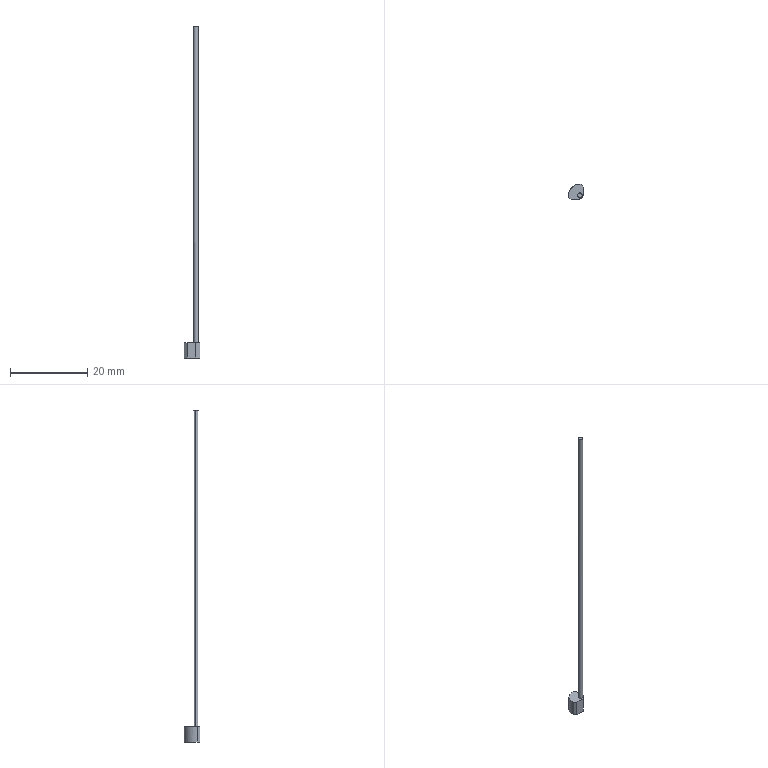Part | Creo | 1 solid | 13 faces | box 4 x 4 x 86.149 mm | volume 144.445 mm3 | plane 8 | cylinder 3 | cone 2 | commonest cylinder face diameters 1.2 x2 6 x1
STEP:
#1=CARTESIAN_POINT('',(0.,0.,0.));
#2=DIRECTION('',(0.,0.,1.));
#3=DIRECTION('',(1.,0.,0.));
#4=AXIS2_PLACEMENT_3D('',#1,#2,#3);
#5=CARTESIAN_POINT('',(29.569,-76.905,32.05));
#6=VERTEX_POINT('',#5);
#7=CARTESIAN_POINT('',(28.969,-77.496,32.059));
#8=VERTEX_POINT('',#7);
#9=CARTESIAN_POINT('',(29.569,-77.496,32.059));
#10=DIRECTION('',(0.,0.,1.));
#11=DIRECTION('',(-0.000001887,1.,0.));
#12=AXIS2_PLACEMENT_3D('',#9,#10,#11);
#13=CIRCLE('',#12,0.6);
#14=EDGE_CURVE('',#6,#8,#13,.T.);
#15=ORIENTED_EDGE('',*,*,#14,.T.);
#16=CARTESIAN_POINT('',(28.969,-77.496,-50.09));
#17=VERTEX_POINT('',#16);
#18=CARTESIAN_POINT('',(28.969,-77.496,32.059));
#19=DIRECTION('',(0.,0.,-1.));
#20=VECTOR('',#19,82.149);
#21=LINE('',#18,#20);
#22=EDGE_CURVE('',#8,#17,#21,.T.);
#23=ORIENTED_EDGE('',*,*,#22,.T.);
#24=CARTESIAN_POINT('',(30.169,-77.496,-50.09));
#25=VERTEX_POINT('',#24);
#26=CARTESIAN_POINT('',(29.569,-77.496,-50.09));
#27=DIRECTION('',(0.,0.,-1.));
#28=DIRECTION('',(-1.,0.,0.));
#29=AXIS2_PLACEMENT_3D('',#26,#27,#28);
#30=CIRCLE('',#29,0.6);
#31=EDGE_CURVE('',#17,#25,#30,.T.);
#32=ORIENTED_EDGE('',*,*,#31,.T.);
#33=CARTESIAN_POINT('',(30.169,-77.496,32.059));
#34=VERTEX_POINT('',#33);
#35=CARTESIAN_POINT('',(30.169,-77.496,32.059));
#36=DIRECTION('',(0.,0.,-1.));
#37=VECTOR('',#36,82.149);
#38=LINE('',#35,#37);
#39=EDGE_CURVE('',#34,#25,#38,.T.);
#40=ORIENTED_EDGE('',*,*,#39,.F.);
#41=CARTESIAN_POINT('',(29.569,-77.496,32.059));
#42=DIRECTION('',(0.,0.,1.));
#43=DIRECTION('',(1.,0.,0.));
#44=AXIS2_PLACEMENT_3D('',#41,#42,#43);
#45=CIRCLE('',#44,0.6);
#46=EDGE_CURVE('',#34,#6,#45,.T.);
#47=ORIENTED_EDGE('',*,*,#46,.T.);
#48=EDGE_LOOP('',(#15,#23,#32,#40,#47));
#49=FACE_OUTER_BOUND('',#48,.F.);
#50=CARTESIAN_POINT('',(29.569,-77.496,32.041));
#51=DIRECTION('',(0.,0.,-1.));
#52=DIRECTION('',(-1.,0.,0.));
#53=AXIS2_PLACEMENT_3D('',#50,#51,#52);
#54=CYLINDRICAL_SURFACE('',#53,0.6);
#55=ADVANCED_FACE('',(#49),#54,.T.);
#56=ORIENTED_EDGE('',*,*,#14,.F.);
#57=CARTESIAN_POINT('',(29.569,-78.087,32.05));
#58=VERTEX_POINT('',#57);
#59=CARTESIAN_POINT('',(29.569,-76.905,32.05));
#60=CARTESIAN_POINT('',(29.498,-76.905,32.05));
#61=CARTESIAN_POINT('',(29.366,-76.943,32.037));
#62=CARTESIAN_POINT('',(29.187,-77.041,32.042));
#63=CARTESIAN_POINT('',(29.057,-77.198,32.041));
#64=CARTESIAN_POINT('',(28.985,-77.391,32.041));
#65=CARTESIAN_POINT('',(28.984,-77.597,32.041));
#66=CARTESIAN_POINT('',(29.054,-77.79,32.041));
#67=CARTESIAN_POINT('',(29.184,-77.949,32.042));
#68=CARTESIAN_POINT('',(29.366,-78.049,32.037));
#69=CARTESIAN_POINT('',(29.498,-78.087,32.05));
#70=CARTESIAN_POINT('',(29.569,-78.087,32.05));
#71=B_SPLINE_CURVE_WITH_KNOTS('',3,(#59,#60,#61,#62,#63,#64,#65,#66,#67,#68,#69,#70),.UNSPECIFIED.,.F.,.F.,(4,1,1,1,1,1,1,1,1,4),(0.,0.1111,0.2222,0.3333,0.4444,0.5556,0.6667,0.7778,0.8889,1.),.UNSPECIFIED.);
#72=EDGE_CURVE('',#6,#58,#71,.T.);
#73=ORIENTED_EDGE('',*,*,#72,.T.);
#74=CARTESIAN_POINT('',(29.569,-77.496,32.059));
#75=DIRECTION('',(0.,0.,1.));
#76=DIRECTION('',(-1.,0.,0.));
#77=AXIS2_PLACEMENT_3D('',#74,#75,#76);
#78=CIRCLE('',#77,0.6);
#79=EDGE_CURVE('',#8,#58,#78,.T.);
#80=ORIENTED_EDGE('',*,*,#79,.F.);
#81=EDGE_LOOP('',(#56,#73,#80));
#82=FACE_OUTER_BOUND('',#81,.F.);
#83=CARTESIAN_POINT('',(29.569,-77.496,32.05));
#84=DIRECTION('',(0.,0.,1.));
#85=DIRECTION('',(-1.,0.,0.));
#86=AXIS2_PLACEMENT_3D('',#83,#84,#85);
#87=CONICAL_SURFACE('',#86,0.5907,45.637);
#88=ADVANCED_FACE('',(#82),#87,.F.);
#89=ORIENTED_EDGE('',*,*,#72,.F.);
#90=CARTESIAN_POINT('',(30.151,-77.496,32.041));
#91=VERTEX_POINT('',#90);
#92=CARTESIAN_POINT('',(30.151,-77.496,32.041));
#93=CARTESIAN_POINT('',(30.151,-77.433,32.041));
#94=CARTESIAN_POINT('',(30.131,-77.313,32.041));
#95=CARTESIAN_POINT('',(30.047,-77.148,32.041));
#96=CARTESIAN_POINT('',(29.917,-77.017,32.042));
#97=CARTESIAN_POINT('',(29.752,-76.938,32.037));
#98=CARTESIAN_POINT('',(29.632,-76.905,32.05));
#99=B_SPLINE_CURVE_WITH_KNOTS('',3,(#92,#93,#94,#95,#96,#97,#98,#5),.UNSPECIFIED.,.F.,.F.,(4,1,1,1,1,4),(0.,0.2,0.4,0.6,0.8,1.),.UNSPECIFIED.);
#100=EDGE_CURVE('',#91,#6,#99,.T.);
#101=ORIENTED_EDGE('',*,*,#100,.F.);
#102=CARTESIAN_POINT('',(29.632,-78.087,32.05));
#103=CARTESIAN_POINT('',(29.752,-78.054,32.037));
#104=CARTESIAN_POINT('',(29.917,-77.975,32.042));
#105=CARTESIAN_POINT('',(30.047,-77.844,32.041));
#106=CARTESIAN_POINT('',(30.131,-77.679,32.041));
#107=CARTESIAN_POINT('',(30.151,-77.559,32.041));
#108=B_SPLINE_CURVE_WITH_KNOTS('',3,(#57,#102,#103,#104,#105,#106,#107,#90),.UNSPECIFIED.,.F.,.F.,(4,1,1,1,1,4),(0.,0.2,0.4,0.6,0.8,1.),.UNSPECIFIED.);
#109=EDGE_CURVE('',#58,#91,#108,.T.);
#110=ORIENTED_EDGE('',*,*,#109,.F.);
#111=EDGE_LOOP('',(#89,#101,#110));
#112=FACE_OUTER_BOUND('',#111,.F.);
#113=CARTESIAN_POINT('',(-0.07825,-88.35,32.041));
#114=DIRECTION('',(0.,0.,-1.));
#115=DIRECTION('',(0.,-1.,0.));
#116=AXIS2_PLACEMENT_3D('',#113,#114,#115);
#117=PLANE('',#116);
#118=ADVANCED_FACE('',(#112),#117,.F.);
#119=ORIENTED_EDGE('',*,*,#46,.F.);
#120=CARTESIAN_POINT('',(29.569,-77.496,32.059));
#121=DIRECTION('',(0.,0.,1.));
#122=DIRECTION('',(0.000001887,-1.,0.));
#123=AXIS2_PLACEMENT_3D('',#120,#121,#122);
#124=CIRCLE('',#123,0.6);
#125=EDGE_CURVE('',#58,#34,#124,.T.);
#126=ORIENTED_EDGE('',*,*,#125,.F.);
#127=ORIENTED_EDGE('',*,*,#109,.T.);
#128=ORIENTED_EDGE('',*,*,#100,.T.);
#129=EDGE_LOOP('',(#119,#126,#127,#128));
#130=FACE_OUTER_BOUND('',#129,.F.);
#131=CARTESIAN_POINT('',(29.569,-77.496,32.05));
#132=DIRECTION('',(0.,0.,1.));
#133=DIRECTION('',(-1.,0.,0.));
#134=AXIS2_PLACEMENT_3D('',#131,#132,#133);
#135=CONICAL_SURFACE('',#134,0.5907,45.637);
#136=ADVANCED_FACE('',(#130),#135,.F.);
#137=ORIENTED_EDGE('',*,*,#79,.T.);
#138=ORIENTED_EDGE('',*,*,#125,.T.);
#139=ORIENTED_EDGE('',*,*,#39,.T.);
#140=CARTESIAN_POINT('',(29.569,-77.496,-50.09));
#141=DIRECTION('',(0.,0.,-1.));
#142=DIRECTION('',(1.,0.,0.));
#143=AXIS2_PLACEMENT_3D('',#140,#141,#142);
#144=CIRCLE('',#143,0.6);
#145=EDGE_CURVE('',#25,#17,#144,.T.);
#146=ORIENTED_EDGE('',*,*,#145,.T.);
#147=ORIENTED_EDGE('',*,*,#22,.F.);
#148=EDGE_LOOP('',(#137,#138,#139,#146,#147));
#149=FACE_OUTER_BOUND('',#148,.F.);
#150=CARTESIAN_POINT('',(29.569,-77.496,32.041));
#151=DIRECTION('',(0.,0.,-1.));
#152=DIRECTION('',(-1.,0.,0.));
#153=AXIS2_PLACEMENT_3D('',#150,#151,#152);
#154=CYLINDRICAL_SURFACE('',#153,0.6);
#155=ADVANCED_FACE('',(#149),#154,.T.);
#156=CARTESIAN_POINT('',(29.952,-74.521,-50.09));
#157=VERTEX_POINT('',#156);
#158=CARTESIAN_POINT('',(26.569,-77.496,-50.09));
#159=VERTEX_POINT('',#158);
#160=CARTESIAN_POINT('',(29.569,-77.496,-50.09));
#161=DIRECTION('',(0.,0.,1.));
#162=DIRECTION('',(0.1277,0.9918,0.));
#163=AXIS2_PLACEMENT_3D('',#160,#161,#162);
#164=CIRCLE('',#163,3.);
#165=EDGE_CURVE('',#157,#159,#164,.T.);
#166=ORIENTED_EDGE('',*,*,#165,.F.);
#167=CARTESIAN_POINT('',(30.569,-75.222,-50.09));
#168=VERTEX_POINT('',#167);
#169=CARTESIAN_POINT('',(30.569,-75.222,-50.09));
#170=DIRECTION('',(-0.6604,0.7509,0.));
#171=VECTOR('',#170,0.9339);
#172=LINE('',#169,#171);
#173=EDGE_CURVE('',#168,#157,#172,.T.);
#174=ORIENTED_EDGE('',*,*,#173,.F.);
#175=CARTESIAN_POINT('',(30.569,-77.496,-50.09));
#176=VERTEX_POINT('',#175);
#177=CARTESIAN_POINT('',(30.569,-75.222,-50.09));
#178=DIRECTION('',(0.,-1.,0.));
#179=VECTOR('',#178,2.274);
#180=LINE('',#177,#179);
#181=EDGE_CURVE('',#168,#176,#180,.T.);
#182=ORIENTED_EDGE('',*,*,#181,.T.);
#183=CARTESIAN_POINT('',(29.569,-78.496,-50.09));
#184=VERTEX_POINT('',#183);
#185=CARTESIAN_POINT('',(29.569,-78.496,-50.09));
#186=DIRECTION('',(0.7071,0.7071,0.));
#187=VECTOR('',#186,1.414);
#188=LINE('',#185,#187);
#189=EDGE_CURVE('',#184,#176,#188,.T.);
#190=ORIENTED_EDGE('',*,*,#189,.F.);
#191=CARTESIAN_POINT('',(27.295,-78.496,-50.09));
#192=VERTEX_POINT('',#191);
#193=CARTESIAN_POINT('',(27.295,-78.496,-50.09));
#194=DIRECTION('',(1.,0.,0.));
#195=VECTOR('',#194,2.274);
#196=LINE('',#193,#195);
#197=EDGE_CURVE('',#192,#184,#196,.T.);
#198=ORIENTED_EDGE('',*,*,#197,.F.);
#199=CARTESIAN_POINT('',(26.594,-77.879,-50.09));
#200=VERTEX_POINT('',#199);
#201=CARTESIAN_POINT('',(26.594,-77.879,-50.09));
#202=DIRECTION('',(0.7509,-0.6604,0.));
#203=VECTOR('',#202,0.9339);
#204=LINE('',#201,#203);
#205=EDGE_CURVE('',#200,#192,#204,.T.);
#206=ORIENTED_EDGE('',*,*,#205,.F.);
#207=CARTESIAN_POINT('',(29.569,-77.496,-50.09));
#208=DIRECTION('',(0.,0.,1.));
#209=DIRECTION('',(-1.,0.,0.));
#210=AXIS2_PLACEMENT_3D('',#207,#208,#209);
#211=CIRCLE('',#210,3.);
#212=EDGE_CURVE('',#159,#200,#211,.T.);
#213=ORIENTED_EDGE('',*,*,#212,.F.);
#214=EDGE_LOOP('',(#166,#174,#182,#190,#198,#206,#213));
#215=FACE_OUTER_BOUND('',#214,.F.);
#216=ORIENTED_EDGE('',*,*,#145,.F.);
#217=ORIENTED_EDGE('',*,*,#31,.F.);
#218=EDGE_LOOP('',(#216,#217));
#219=FACE_BOUND('',#218,.F.);
#220=CARTESIAN_POINT('',(26.741,-78.496,-50.09));
#221=DIRECTION('',(0.,0.,1.));
#222=DIRECTION('',(1.,0.,0.));
#223=AXIS2_PLACEMENT_3D('',#220,#221,#222);
#224=PLANE('',#223);
#225=ADVANCED_FACE('',(#215,#219),#224,.T.);
#226=CARTESIAN_POINT('',(26.594,-77.879,-54.09));
#227=VERTEX_POINT('',#226);
#228=CARTESIAN_POINT('',(29.952,-74.521,-54.09));
#229=VERTEX_POINT('',#228);
#230=CARTESIAN_POINT('',(29.569,-77.496,-54.09));
#231=DIRECTION('',(0.,0.,-1.));
#232=DIRECTION('',(-0.9918,-0.1277,0.));
#233=AXIS2_PLACEMENT_3D('',#230,#231,#232);
#234=CIRCLE('',#233,3.);
#235=EDGE_CURVE('',#227,#229,#234,.T.);
#236=ORIENTED_EDGE('',*,*,#235,.T.);
#237=CARTESIAN_POINT('',(29.952,-74.521,-50.09));
#238=DIRECTION('',(0.,0.,-1.));
#239=VECTOR('',#238,4.);
#240=LINE('',#237,#239);
#241=EDGE_CURVE('',#157,#229,#240,.T.);
#242=ORIENTED_EDGE('',*,*,#241,.F.);
#243=ORIENTED_EDGE('',*,*,#165,.T.);
#244=ORIENTED_EDGE('',*,*,#212,.T.);
#245=CARTESIAN_POINT('',(26.594,-77.879,-54.09));
#246=DIRECTION('',(0.,0.,1.));
#247=VECTOR('',#246,4.);
#248=LINE('',#245,#247);
#249=EDGE_CURVE('',#227,#200,#248,.T.);
#250=ORIENTED_EDGE('',*,*,#249,.F.);
#251=EDGE_LOOP('',(#236,#242,#243,#244,#250));
#252=FACE_OUTER_BOUND('',#251,.F.);
#253=CARTESIAN_POINT('',(29.569,-77.496,-44.09));
#254=DIRECTION('',(0.,0.,1.));
#255=DIRECTION('',(1.,0.,0.));
#256=AXIS2_PLACEMENT_3D('',#253,#254,#255);
#257=CYLINDRICAL_SURFACE('',#256,3.);
#258=ADVANCED_FACE('',(#252),#257,.T.);
#259=CARTESIAN_POINT('',(27.295,-78.496,-54.09));
#260=VERTEX_POINT('',#259);
#261=CARTESIAN_POINT('',(29.569,-78.496,-54.09));
#262=VERTEX_POINT('',#261);
#263=CARTESIAN_POINT('',(27.295,-78.496,-54.09));
#264=DIRECTION('',(1.,0.,0.));
#265=VECTOR('',#264,2.274);
#266=LINE('',#263,#265);
#267=EDGE_CURVE('',#260,#262,#266,.T.);
#268=ORIENTED_EDGE('',*,*,#267,.T.);
#269=CARTESIAN_POINT('',(30.569,-77.496,-54.09));
#270=VERTEX_POINT('',#269);
#271=CARTESIAN_POINT('',(30.569,-77.496,-54.09));
#272=DIRECTION('',(-0.7071,-0.7071,0.));
#273=VECTOR('',#272,1.414);
#274=LINE('',#271,#273);
#275=EDGE_CURVE('',#270,#262,#274,.T.);
#276=ORIENTED_EDGE('',*,*,#275,.F.);
#277=CARTESIAN_POINT('',(30.569,-75.222,-54.09));
#278=VERTEX_POINT('',#277);
#279=CARTESIAN_POINT('',(30.569,-77.496,-54.09));
#280=DIRECTION('',(0.,1.,0.));
#281=VECTOR('',#280,2.274);
#282=LINE('',#279,#281);
#283=EDGE_CURVE('',#270,#278,#282,.T.);
#284=ORIENTED_EDGE('',*,*,#283,.T.);
#285=CARTESIAN_POINT('',(29.952,-74.521,-54.09));
#286=DIRECTION('',(0.6604,-0.7509,0.));
#287=VECTOR('',#286,0.9339);
#288=LINE('',#285,#287);
#289=EDGE_CURVE('',#229,#278,#288,.T.);
#290=ORIENTED_EDGE('',*,*,#289,.F.);
#291=ORIENTED_EDGE('',*,*,#235,.F.);
#292=CARTESIAN_POINT('',(27.295,-78.496,-54.09));
#293=DIRECTION('',(-0.7509,0.6604,0.));
#294=VECTOR('',#293,0.9339);
#295=LINE('',#292,#294);
#296=EDGE_CURVE('',#260,#227,#295,.T.);
#297=ORIENTED_EDGE('',*,*,#296,.F.);
#298=EDGE_LOOP('',(#268,#276,#284,#290,#291,#297));
#299=FACE_OUTER_BOUND('',#298,.F.);
#300=CARTESIAN_POINT('',(0.,0.,-54.09));
#301=DIRECTION('',(0.,0.,-1.));
#302=DIRECTION('',(-1.,0.,0.));
#303=AXIS2_PLACEMENT_3D('',#300,#301,#302);
#304=PLANE('',#303);
#305=ADVANCED_FACE('',(#299),#304,.T.);
#306=ORIENTED_EDGE('',*,*,#197,.T.);
#307=CARTESIAN_POINT('',(29.569,-78.496,-50.09));
#308=DIRECTION('',(0.,0.,-1.));
#309=VECTOR('',#308,4.);
#310=LINE('',#307,#309);
#311=EDGE_CURVE('',#184,#262,#310,.T.);
#312=ORIENTED_EDGE('',*,*,#311,.T.);
#313=ORIENTED_EDGE('',*,*,#267,.F.);
#314=CARTESIAN_POINT('',(27.295,-78.496,-54.09));
#315=DIRECTION('',(0.,0.,1.));
#316=VECTOR('',#315,4.);
#317=LINE('',#314,#316);
#318=EDGE_CURVE('',#260,#192,#317,.T.);
#319=ORIENTED_EDGE('',*,*,#318,.T.);
#320=EDGE_LOOP('',(#306,#312,#313,#319));
#321=FACE_OUTER_BOUND('',#320,.F.);
#322=CARTESIAN_POINT('',(30.569,-78.496,-44.09));
#323=DIRECTION('',(0.,1.,0.));
#324=DIRECTION('',(0.,0.,1.));
#325=AXIS2_PLACEMENT_3D('',#322,#323,#324);
#326=PLANE('',#325);
#327=ADVANCED_FACE('',(#321),#326,.F.);
#328=ORIENTED_EDGE('',*,*,#275,.T.);
#329=ORIENTED_EDGE('',*,*,#311,.F.);
#330=ORIENTED_EDGE('',*,*,#189,.T.);
#331=CARTESIAN_POINT('',(30.569,-77.496,-54.09));
#332=DIRECTION('',(0.,0.,1.));
#333=VECTOR('',#332,4.);
#334=LINE('',#331,#333);
#335=EDGE_CURVE('',#270,#176,#334,.T.);
#336=ORIENTED_EDGE('',*,*,#335,.F.);
#337=EDGE_LOOP('',(#328,#329,#330,#336));
#338=FACE_OUTER_BOUND('',#337,.F.);
#339=CARTESIAN_POINT('',(29.569,-78.496,-44.09));
#340=DIRECTION('',(0.7071,-0.7071,0.));
#341=DIRECTION('',(0.,0.,-1.));
#342=AXIS2_PLACEMENT_3D('',#339,#340,#341);
#343=PLANE('',#342);
#344=ADVANCED_FACE('',(#338),#343,.T.);
#345=ORIENTED_EDGE('',*,*,#283,.F.);
#346=ORIENTED_EDGE('',*,*,#335,.T.);
#347=ORIENTED_EDGE('',*,*,#181,.F.);
#348=CARTESIAN_POINT('',(30.569,-75.222,-50.09));
#349=DIRECTION('',(0.,0.,-1.));
#350=VECTOR('',#349,4.);
#351=LINE('',#348,#350);
#352=EDGE_CURVE('',#168,#278,#351,.T.);
#353=ORIENTED_EDGE('',*,*,#352,.T.);
#354=EDGE_LOOP('',(#345,#346,#347,#353));
#355=FACE_OUTER_BOUND('',#354,.F.);
#356=CARTESIAN_POINT('',(30.569,-77.496,-44.09));
#357=DIRECTION('',(1.,0.,0.));
#358=DIRECTION('',(0.,0.,-1.));
#359=AXIS2_PLACEMENT_3D('',#356,#357,#358);
#360=PLANE('',#359);
#361=ADVANCED_FACE('',(#355),#360,.T.);
#362=ORIENTED_EDGE('',*,*,#173,.T.);
#363=ORIENTED_EDGE('',*,*,#241,.T.);
#364=ORIENTED_EDGE('',*,*,#289,.T.);
#365=ORIENTED_EDGE('',*,*,#352,.F.);
#366=EDGE_LOOP('',(#362,#363,#364,#365));
#367=FACE_OUTER_BOUND('',#366,.F.);
#368=CARTESIAN_POINT('',(29.952,-74.521,-44.09));
#369=DIRECTION('',(0.7509,0.6604,0.));
#370=DIRECTION('',(0.,0.,1.));
#371=AXIS2_PLACEMENT_3D('',#368,#369,#370);
#372=PLANE('',#371);
#373=ADVANCED_FACE('',(#367),#372,.T.);
#374=ORIENTED_EDGE('',*,*,#296,.T.);
#375=ORIENTED_EDGE('',*,*,#249,.T.);
#376=ORIENTED_EDGE('',*,*,#205,.T.);
#377=ORIENTED_EDGE('',*,*,#318,.F.);
#378=EDGE_LOOP('',(#374,#375,#376,#377));
#379=FACE_OUTER_BOUND('',#378,.F.);
#380=CARTESIAN_POINT('',(26.594,-77.879,-44.09));
#381=DIRECTION('',(0.6604,0.7509,0.));
#382=DIRECTION('',(0.,0.,1.));
#383=AXIS2_PLACEMENT_3D('',#380,#381,#382);
#384=PLANE('',#383);
#385=ADVANCED_FACE('',(#379),#384,.F.);
#386=CLOSED_SHELL('',(#55,#88,#118,#136,#155,#225,#258,#305,#327,#344,#361,#373,#385));
#387=MANIFOLD_SOLID_BREP('',#386);
#388=(LENGTH_UNIT()NAMED_UNIT(*)SI_UNIT(.MILLI.,.METRE.));
#389=UNCERTAINTY_MEASURE_WITH_UNIT(LENGTH_MEASURE(0.01298),#388,'','');
#390=(NAMED_UNIT(*)PLANE_ANGLE_UNIT()SI_UNIT($,.RADIAN.));
#391=PLANE_ANGLE_MEASURE_WITH_UNIT(PLANE_ANGLE_MEASURE(0.01745),#390);
#392=(CONVERSION_BASED_UNIT('DEGREE',#391)NAMED_UNIT(*)PLANE_ANGLE_UNIT());
#393=(NAMED_UNIT(*)SI_UNIT($,.STERADIAN.)SOLID_ANGLE_UNIT());
#394=(GEOMETRIC_REPRESENTATION_CONTEXT(3)GLOBAL_UNCERTAINTY_ASSIGNED_CONTEXT((#389))GLOBAL_UNIT_ASSIGNED_CONTEXT((#388,#392,#393))REPRESENTATION_CONTEXT('',''));
#395=ADVANCED_BREP_SHAPE_REPRESENTATION('',(#4,#387),#394);